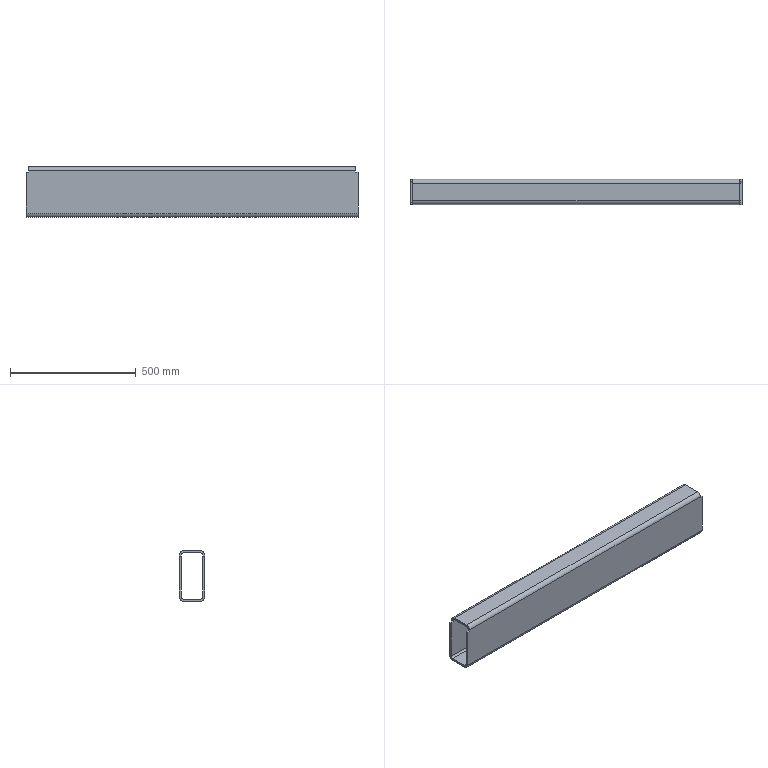Part | SolidWorks | features ICE 1, MirrorPattern 1, WeldMemberFeat 1, WeldmentFeature 1 | 1 solid | 24 faces | box 1321 x 100 x 200 mm | volume 5764189 mm3 | plane 16 | cylinder 8 | commonest cylinder face diameters 16 x4 32 x4
STEP:
#1=CARTESIAN_POINT('',(649.5,50.,84.));
#2=VERTEX_POINT('',#1);
#3=CARTESIAN_POINT('',(649.5,34.,100.));
#4=VERTEX_POINT('',#3);
#5=CARTESIAN_POINT('',(649.5,34.,84.));
#6=DIRECTION('',(1.,0.,0.));
#7=DIRECTION('',(0.,0.,-1.));
#8=AXIS2_PLACEMENT_3D('',#5,#6,#7);
#9=CIRCLE('',#8,16.);
#10=EDGE_CURVE('',#2,#4,#9,.T.);
#11=ORIENTED_EDGE('',*,*,#10,.F.);
#12=CARTESIAN_POINT('',(-649.5,50.,84.));
#13=VERTEX_POINT('',#12);
#14=CARTESIAN_POINT('',(660.5,50.,84.));
#15=DIRECTION('',(-1.,0.,0.));
#16=VECTOR('',#15,1000.);
#17=LINE('',#14,#16);
#18=EDGE_CURVE('',#2,#13,#17,.T.);
#19=ORIENTED_EDGE('',*,*,#18,.T.);
#20=CARTESIAN_POINT('',(-649.5,34.,100.));
#21=VERTEX_POINT('',#20);
#22=CARTESIAN_POINT('',(-649.5,34.,84.));
#23=DIRECTION('',(1.,0.,0.));
#24=DIRECTION('',(0.,0.,-1.));
#25=AXIS2_PLACEMENT_3D('',#22,#23,#24);
#26=CIRCLE('',#25,16.);
#27=EDGE_CURVE('',#13,#21,#26,.T.);
#28=ORIENTED_EDGE('',*,*,#27,.T.);
#29=CARTESIAN_POINT('',(660.5,34.,100.));
#30=DIRECTION('',(-1.,0.,0.));
#31=VECTOR('',#30,1000.);
#32=LINE('',#29,#31);
#33=EDGE_CURVE('',#4,#21,#32,.T.);
#34=ORIENTED_EDGE('',*,*,#33,.F.);
#35=EDGE_LOOP('',(#11,#19,#28,#34));
#36=FACE_OUTER_BOUND('',#35,.T.);
#37=CARTESIAN_POINT('',(660.5,34.,84.));
#38=DIRECTION('',(-1.,0.,0.));
#39=DIRECTION('',(0.,0.,1.));
#40=AXIS2_PLACEMENT_3D('',#37,#38,#39);
#41=CYLINDRICAL_SURFACE('',#40,16.);
#42=ADVANCED_FACE('',(#36),#41,.T.);
#43=CARTESIAN_POINT('',(649.5,-34.,100.));
#44=VERTEX_POINT('',#43);
#45=CARTESIAN_POINT('',(649.5,50.,100.));
#46=DIRECTION('',(0.,-1.,0.));
#47=VECTOR('',#46,1000.);
#48=LINE('',#45,#47);
#49=EDGE_CURVE('',#4,#44,#48,.T.);
#50=ORIENTED_EDGE('',*,*,#49,.F.);
#51=ORIENTED_EDGE('',*,*,#33,.T.);
#52=CARTESIAN_POINT('',(-649.5,-34.,100.));
#53=VERTEX_POINT('',#52);
#54=CARTESIAN_POINT('',(-649.5,50.,100.));
#55=DIRECTION('',(0.,-1.,0.));
#56=VECTOR('',#55,1000.);
#57=LINE('',#54,#56);
#58=EDGE_CURVE('',#21,#53,#57,.T.);
#59=ORIENTED_EDGE('',*,*,#58,.T.);
#60=CARTESIAN_POINT('',(660.5,-34.,100.));
#61=DIRECTION('',(-1.,0.,0.));
#62=VECTOR('',#61,1000.);
#63=LINE('',#60,#62);
#64=EDGE_CURVE('',#44,#53,#63,.T.);
#65=ORIENTED_EDGE('',*,*,#64,.F.);
#66=EDGE_LOOP('',(#50,#51,#59,#65));
#67=FACE_OUTER_BOUND('',#66,.T.);
#68=CARTESIAN_POINT('',(660.5,34.,100.));
#69=DIRECTION('',(0.,0.,-1.));
#70=DIRECTION('',(-1.,0.,0.));
#71=AXIS2_PLACEMENT_3D('',#68,#69,#70);
#72=PLANE('',#71);
#73=ADVANCED_FACE('',(#67),#72,.F.);
#74=CARTESIAN_POINT('',(649.5,-50.,84.));
#75=VERTEX_POINT('',#74);
#76=CARTESIAN_POINT('',(649.5,-34.,84.));
#77=DIRECTION('',(1.,0.,0.));
#78=DIRECTION('',(0.,0.,-1.));
#79=AXIS2_PLACEMENT_3D('',#76,#77,#78);
#80=CIRCLE('',#79,16.);
#81=EDGE_CURVE('',#44,#75,#80,.T.);
#82=ORIENTED_EDGE('',*,*,#81,.F.);
#83=ORIENTED_EDGE('',*,*,#64,.T.);
#84=CARTESIAN_POINT('',(-649.5,-50.,84.));
#85=VERTEX_POINT('',#84);
#86=CARTESIAN_POINT('',(-649.5,-34.,84.));
#87=DIRECTION('',(1.,0.,0.));
#88=DIRECTION('',(0.,0.,-1.));
#89=AXIS2_PLACEMENT_3D('',#86,#87,#88);
#90=CIRCLE('',#89,16.);
#91=EDGE_CURVE('',#53,#85,#90,.T.);
#92=ORIENTED_EDGE('',*,*,#91,.T.);
#93=CARTESIAN_POINT('',(660.5,-50.,84.));
#94=DIRECTION('',(-1.,0.,0.));
#95=VECTOR('',#94,1000.);
#96=LINE('',#93,#95);
#97=EDGE_CURVE('',#75,#85,#96,.T.);
#98=ORIENTED_EDGE('',*,*,#97,.F.);
#99=EDGE_LOOP('',(#82,#83,#92,#98));
#100=FACE_OUTER_BOUND('',#99,.T.);
#101=CARTESIAN_POINT('',(660.5,-34.,84.));
#102=DIRECTION('',(-1.,0.,0.));
#103=DIRECTION('',(0.,0.,1.));
#104=AXIS2_PLACEMENT_3D('',#101,#102,#103);
#105=CYLINDRICAL_SURFACE('',#104,16.);
#106=ADVANCED_FACE('',(#100),#105,.T.);
#107=CARTESIAN_POINT('',(660.5,-50.,78.));
#108=VERTEX_POINT('',#107);
#109=CARTESIAN_POINT('',(649.5,-50.,78.));
#110=VERTEX_POINT('',#109);
#111=CARTESIAN_POINT('',(660.5,-50.,78.));
#112=DIRECTION('',(-1.,0.,0.));
#113=VECTOR('',#112,1000.);
#114=LINE('',#111,#113);
#115=EDGE_CURVE('',#108,#110,#114,.T.);
#116=ORIENTED_EDGE('',*,*,#115,.T.);
#117=CARTESIAN_POINT('',(649.5,-50.,100.));
#118=DIRECTION('',(0.,0.,1.));
#119=VECTOR('',#118,1000.);
#120=LINE('',#117,#119);
#121=EDGE_CURVE('',#110,#75,#120,.T.);
#122=ORIENTED_EDGE('',*,*,#121,.T.);
#123=ORIENTED_EDGE('',*,*,#97,.T.);
#124=CARTESIAN_POINT('',(-649.5,-50.,78.));
#125=VERTEX_POINT('',#124);
#126=CARTESIAN_POINT('',(-649.5,-50.,100.));
#127=DIRECTION('',(0.,0.,1.));
#128=VECTOR('',#127,1000.);
#129=LINE('',#126,#128);
#130=EDGE_CURVE('',#125,#85,#129,.T.);
#131=ORIENTED_EDGE('',*,*,#130,.F.);
#132=CARTESIAN_POINT('',(-660.5,-50.,78.));
#133=VERTEX_POINT('',#132);
#134=CARTESIAN_POINT('',(-660.5,-50.,78.));
#135=DIRECTION('',(1.,0.,0.));
#136=VECTOR('',#135,1000.);
#137=LINE('',#134,#136);
#138=EDGE_CURVE('',#133,#125,#137,.T.);
#139=ORIENTED_EDGE('',*,*,#138,.F.);
#140=CARTESIAN_POINT('',(-660.5,-50.,-84.));
#141=VERTEX_POINT('',#140);
#142=CARTESIAN_POINT('',(-660.5,-50.,-84.));
#143=DIRECTION('',(0.,0.,-1.));
#144=VECTOR('',#143,1000.);
#145=LINE('',#142,#144);
#146=EDGE_CURVE('',#133,#141,#145,.T.);
#147=ORIENTED_EDGE('',*,*,#146,.T.);
#148=CARTESIAN_POINT('',(660.5,-50.,-84.));
#149=VERTEX_POINT('',#148);
#150=CARTESIAN_POINT('',(660.5,-50.,-84.));
#151=DIRECTION('',(-1.,0.,0.));
#152=VECTOR('',#151,1000.);
#153=LINE('',#150,#152);
#154=EDGE_CURVE('',#149,#141,#153,.T.);
#155=ORIENTED_EDGE('',*,*,#154,.F.);
#156=CARTESIAN_POINT('',(660.5,-50.,-84.));
#157=DIRECTION('',(0.,0.,-1.));
#158=VECTOR('',#157,1000.);
#159=LINE('',#156,#158);
#160=EDGE_CURVE('',#108,#149,#159,.T.);
#161=ORIENTED_EDGE('',*,*,#160,.F.);
#162=EDGE_LOOP('',(#116,#122,#123,#131,#139,#147,#155,#161));
#163=FACE_OUTER_BOUND('',#162,.T.);
#164=CARTESIAN_POINT('',(660.5,-50.,-84.));
#165=DIRECTION('',(0.,1.,0.));
#166=DIRECTION('',(0.,0.,1.));
#167=AXIS2_PLACEMENT_3D('',#164,#165,#166);
#168=PLANE('',#167);
#169=ADVANCED_FACE('',(#163),#168,.F.);
#170=CARTESIAN_POINT('',(649.5,-34.,92.));
#171=VERTEX_POINT('',#170);
#172=CARTESIAN_POINT('',(-649.5,-34.,92.));
#173=VERTEX_POINT('',#172);
#174=CARTESIAN_POINT('',(660.5,-34.,92.));
#175=DIRECTION('',(-1.,0.,0.));
#176=VECTOR('',#175,1000.);
#177=LINE('',#174,#176);
#178=EDGE_CURVE('',#171,#173,#177,.T.);
#179=ORIENTED_EDGE('',*,*,#178,.F.);
#180=CARTESIAN_POINT('',(649.5,-42.,84.));
#181=VERTEX_POINT('',#180);
#182=CARTESIAN_POINT('',(649.5,-34.,84.));
#183=DIRECTION('',(1.,0.,0.));
#184=DIRECTION('',(0.,0.,-1.));
#185=AXIS2_PLACEMENT_3D('',#182,#183,#184);
#186=CIRCLE('',#185,8.);
#187=EDGE_CURVE('',#171,#181,#186,.T.);
#188=ORIENTED_EDGE('',*,*,#187,.T.);
#189=CARTESIAN_POINT('',(-649.5,-42.,84.));
#190=VERTEX_POINT('',#189);
#191=CARTESIAN_POINT('',(660.5,-42.,84.));
#192=DIRECTION('',(-1.,0.,0.));
#193=VECTOR('',#192,1000.);
#194=LINE('',#191,#193);
#195=EDGE_CURVE('',#181,#190,#194,.T.);
#196=ORIENTED_EDGE('',*,*,#195,.T.);
#197=CARTESIAN_POINT('',(-649.5,-34.,84.));
#198=DIRECTION('',(1.,0.,0.));
#199=DIRECTION('',(0.,0.,-1.));
#200=AXIS2_PLACEMENT_3D('',#197,#198,#199);
#201=CIRCLE('',#200,8.);
#202=EDGE_CURVE('',#173,#190,#201,.T.);
#203=ORIENTED_EDGE('',*,*,#202,.F.);
#204=EDGE_LOOP('',(#179,#188,#196,#203));
#205=FACE_OUTER_BOUND('',#204,.T.);
#206=CARTESIAN_POINT('',(660.5,-34.,84.));
#207=DIRECTION('',(-1.,0.,0.));
#208=DIRECTION('',(0.,0.,1.));
#209=AXIS2_PLACEMENT_3D('',#206,#207,#208);
#210=CYLINDRICAL_SURFACE('',#209,8.);
#211=ADVANCED_FACE('',(#205),#210,.F.);
#212=CARTESIAN_POINT('',(649.5,34.,92.));
#213=VERTEX_POINT('',#212);
#214=CARTESIAN_POINT('',(-649.5,34.,92.));
#215=VERTEX_POINT('',#214);
#216=CARTESIAN_POINT('',(660.5,34.,92.));
#217=DIRECTION('',(-1.,0.,0.));
#218=VECTOR('',#217,1000.);
#219=LINE('',#216,#218);
#220=EDGE_CURVE('',#213,#215,#219,.T.);
#221=ORIENTED_EDGE('',*,*,#220,.F.);
#222=CARTESIAN_POINT('',(649.5,34.,92.));
#223=DIRECTION('',(0.,-1.,0.));
#224=VECTOR('',#223,1000.);
#225=LINE('',#222,#224);
#226=EDGE_CURVE('',#213,#171,#225,.T.);
#227=ORIENTED_EDGE('',*,*,#226,.T.);
#228=ORIENTED_EDGE('',*,*,#178,.T.);
#229=CARTESIAN_POINT('',(-649.5,34.,92.));
#230=DIRECTION('',(0.,-1.,0.));
#231=VECTOR('',#230,1000.);
#232=LINE('',#229,#231);
#233=EDGE_CURVE('',#215,#173,#232,.T.);
#234=ORIENTED_EDGE('',*,*,#233,.F.);
#235=EDGE_LOOP('',(#221,#227,#228,#234));
#236=FACE_OUTER_BOUND('',#235,.T.);
#237=CARTESIAN_POINT('',(660.5,34.,92.));
#238=DIRECTION('',(0.,0.,-1.));
#239=DIRECTION('',(-1.,0.,0.));
#240=AXIS2_PLACEMENT_3D('',#237,#238,#239);
#241=PLANE('',#240);
#242=ADVANCED_FACE('',(#236),#241,.T.);
#243=CARTESIAN_POINT('',(649.5,42.,84.));
#244=VERTEX_POINT('',#243);
#245=CARTESIAN_POINT('',(-649.5,42.,84.));
#246=VERTEX_POINT('',#245);
#247=CARTESIAN_POINT('',(660.5,42.,84.));
#248=DIRECTION('',(-1.,0.,0.));
#249=VECTOR('',#248,1000.);
#250=LINE('',#247,#249);
#251=EDGE_CURVE('',#244,#246,#250,.T.);
#252=ORIENTED_EDGE('',*,*,#251,.F.);
#253=CARTESIAN_POINT('',(649.5,34.,84.));
#254=DIRECTION('',(1.,0.,0.));
#255=DIRECTION('',(0.,0.,-1.));
#256=AXIS2_PLACEMENT_3D('',#253,#254,#255);
#257=CIRCLE('',#256,8.);
#258=EDGE_CURVE('',#244,#213,#257,.T.);
#259=ORIENTED_EDGE('',*,*,#258,.T.);
#260=ORIENTED_EDGE('',*,*,#220,.T.);
#261=CARTESIAN_POINT('',(-649.5,34.,84.));
#262=DIRECTION('',(1.,0.,0.));
#263=DIRECTION('',(0.,0.,-1.));
#264=AXIS2_PLACEMENT_3D('',#261,#262,#263);
#265=CIRCLE('',#264,8.);
#266=EDGE_CURVE('',#246,#215,#265,.T.);
#267=ORIENTED_EDGE('',*,*,#266,.F.);
#268=EDGE_LOOP('',(#252,#259,#260,#267));
#269=FACE_OUTER_BOUND('',#268,.T.);
#270=CARTESIAN_POINT('',(660.5,34.,84.));
#271=DIRECTION('',(-1.,0.,0.));
#272=DIRECTION('',(0.,0.,1.));
#273=AXIS2_PLACEMENT_3D('',#270,#271,#272);
#274=CYLINDRICAL_SURFACE('',#273,8.);
#275=ADVANCED_FACE('',(#269),#274,.F.);
#276=CARTESIAN_POINT('',(660.5,42.,-84.));
#277=VERTEX_POINT('',#276);
#278=CARTESIAN_POINT('',(660.5,42.,78.));
#279=VERTEX_POINT('',#278);
#280=CARTESIAN_POINT('',(660.5,42.,84.));
#281=DIRECTION('',(0.,0.,1.));
#282=VECTOR('',#281,1000.);
#283=LINE('',#280,#282);
#284=EDGE_CURVE('',#277,#279,#283,.T.);
#285=ORIENTED_EDGE('',*,*,#284,.T.);
#286=CARTESIAN_POINT('',(649.5,42.,78.));
#287=VERTEX_POINT('',#286);
#288=CARTESIAN_POINT('',(660.5,42.,78.));
#289=DIRECTION('',(-1.,0.,0.));
#290=VECTOR('',#289,1000.);
#291=LINE('',#288,#290);
#292=EDGE_CURVE('',#279,#287,#291,.T.);
#293=ORIENTED_EDGE('',*,*,#292,.T.);
#294=CARTESIAN_POINT('',(649.5,42.,84.));
#295=DIRECTION('',(0.,0.,1.));
#296=VECTOR('',#295,1000.);
#297=LINE('',#294,#296);
#298=EDGE_CURVE('',#287,#244,#297,.T.);
#299=ORIENTED_EDGE('',*,*,#298,.T.);
#300=ORIENTED_EDGE('',*,*,#251,.T.);
#301=CARTESIAN_POINT('',(-649.5,42.,78.));
#302=VERTEX_POINT('',#301);
#303=CARTESIAN_POINT('',(-649.5,42.,84.));
#304=DIRECTION('',(0.,0.,1.));
#305=VECTOR('',#304,1000.);
#306=LINE('',#303,#305);
#307=EDGE_CURVE('',#302,#246,#306,.T.);
#308=ORIENTED_EDGE('',*,*,#307,.F.);
#309=CARTESIAN_POINT('',(-660.5,42.,78.));
#310=VERTEX_POINT('',#309);
#311=CARTESIAN_POINT('',(660.5,42.,78.));
#312=DIRECTION('',(1.,0.,0.));
#313=VECTOR('',#312,1000.);
#314=LINE('',#311,#313);
#315=EDGE_CURVE('',#310,#302,#314,.T.);
#316=ORIENTED_EDGE('',*,*,#315,.F.);
#317=CARTESIAN_POINT('',(-660.5,42.,-84.));
#318=VERTEX_POINT('',#317);
#319=CARTESIAN_POINT('',(-660.5,42.,84.));
#320=DIRECTION('',(0.,0.,1.));
#321=VECTOR('',#320,1000.);
#322=LINE('',#319,#321);
#323=EDGE_CURVE('',#318,#310,#322,.T.);
#324=ORIENTED_EDGE('',*,*,#323,.F.);
#325=CARTESIAN_POINT('',(660.5,42.,-84.));
#326=DIRECTION('',(-1.,0.,0.));
#327=VECTOR('',#326,1000.);
#328=LINE('',#325,#327);
#329=EDGE_CURVE('',#277,#318,#328,.T.);
#330=ORIENTED_EDGE('',*,*,#329,.F.);
#331=EDGE_LOOP('',(#285,#293,#299,#300,#308,#316,#324,#330));
#332=FACE_OUTER_BOUND('',#331,.T.);
#333=CARTESIAN_POINT('',(660.5,42.,84.));
#334=DIRECTION('',(0.,-1.,0.));
#335=DIRECTION('',(0.,0.,-1.));
#336=AXIS2_PLACEMENT_3D('',#333,#334,#335);
#337=PLANE('',#336);
#338=ADVANCED_FACE('',(#332),#337,.T.);
#339=CARTESIAN_POINT('',(649.5,-42.,78.));
#340=VERTEX_POINT('',#339);
#341=CARTESIAN_POINT('',(649.5,-42.,-84.));
#342=DIRECTION('',(0.,0.,-1.));
#343=VECTOR('',#342,1000.);
#344=LINE('',#341,#343);
#345=EDGE_CURVE('',#181,#340,#344,.T.);
#346=ORIENTED_EDGE('',*,*,#345,.T.);
#347=CARTESIAN_POINT('',(660.5,-42.,78.));
#348=VERTEX_POINT('',#347);
#349=CARTESIAN_POINT('',(660.5,-42.,78.));
#350=DIRECTION('',(1.,0.,0.));
#351=VECTOR('',#350,1000.);
#352=LINE('',#349,#351);
#353=EDGE_CURVE('',#340,#348,#352,.T.);
#354=ORIENTED_EDGE('',*,*,#353,.T.);
#355=CARTESIAN_POINT('',(660.5,-42.,-84.));
#356=VERTEX_POINT('',#355);
#357=CARTESIAN_POINT('',(660.5,-42.,-84.));
#358=DIRECTION('',(0.,0.,-1.));
#359=VECTOR('',#358,1000.);
#360=LINE('',#357,#359);
#361=EDGE_CURVE('',#348,#356,#360,.T.);
#362=ORIENTED_EDGE('',*,*,#361,.T.);
#363=CARTESIAN_POINT('',(-660.5,-42.,-84.));
#364=VERTEX_POINT('',#363);
#365=CARTESIAN_POINT('',(660.5,-42.,-84.));
#366=DIRECTION('',(-1.,0.,0.));
#367=VECTOR('',#366,1000.);
#368=LINE('',#365,#367);
#369=EDGE_CURVE('',#356,#364,#368,.T.);
#370=ORIENTED_EDGE('',*,*,#369,.T.);
#371=CARTESIAN_POINT('',(-660.5,-42.,78.));
#372=VERTEX_POINT('',#371);
#373=CARTESIAN_POINT('',(-660.5,-42.,-84.));
#374=DIRECTION('',(0.,0.,-1.));
#375=VECTOR('',#374,1000.);
#376=LINE('',#373,#375);
#377=EDGE_CURVE('',#372,#364,#376,.T.);
#378=ORIENTED_EDGE('',*,*,#377,.F.);
#379=CARTESIAN_POINT('',(-649.5,-42.,78.));
#380=VERTEX_POINT('',#379);
#381=CARTESIAN_POINT('',(660.5,-42.,78.));
#382=DIRECTION('',(-1.,0.,0.));
#383=VECTOR('',#382,1000.);
#384=LINE('',#381,#383);
#385=EDGE_CURVE('',#380,#372,#384,.T.);
#386=ORIENTED_EDGE('',*,*,#385,.F.);
#387=CARTESIAN_POINT('',(-649.5,-42.,-84.));
#388=DIRECTION('',(0.,0.,-1.));
#389=VECTOR('',#388,1000.);
#390=LINE('',#387,#389);
#391=EDGE_CURVE('',#190,#380,#390,.T.);
#392=ORIENTED_EDGE('',*,*,#391,.F.);
#393=ORIENTED_EDGE('',*,*,#195,.F.);
#394=EDGE_LOOP('',(#346,#354,#362,#370,#378,#386,#392,#393));
#395=FACE_OUTER_BOUND('',#394,.T.);
#396=CARTESIAN_POINT('',(660.5,-42.,-84.));
#397=DIRECTION('',(0.,1.,0.));
#398=DIRECTION('',(0.,0.,1.));
#399=AXIS2_PLACEMENT_3D('',#396,#397,#398);
#400=PLANE('',#399);
#401=ADVANCED_FACE('',(#395),#400,.T.);
#402=CARTESIAN_POINT('',(660.5,50.,78.));
#403=VERTEX_POINT('',#402);
#404=CARTESIAN_POINT('',(649.5,50.,78.));
#405=VERTEX_POINT('',#404);
#406=CARTESIAN_POINT('',(660.5,50.,78.));
#407=DIRECTION('',(-1.,0.,0.));
#408=VECTOR('',#407,1000.);
#409=LINE('',#406,#408);
#410=EDGE_CURVE('',#403,#405,#409,.T.);
#411=ORIENTED_EDGE('',*,*,#410,.F.);
#412=CARTESIAN_POINT('',(660.5,50.,-84.));
#413=VERTEX_POINT('',#412);
#414=CARTESIAN_POINT('',(660.5,50.,84.));
#415=DIRECTION('',(0.,0.,1.));
#416=VECTOR('',#415,1000.);
#417=LINE('',#414,#416);
#418=EDGE_CURVE('',#413,#403,#417,.T.);
#419=ORIENTED_EDGE('',*,*,#418,.F.);
#420=CARTESIAN_POINT('',(-660.5,50.,-84.));
#421=VERTEX_POINT('',#420);
#422=CARTESIAN_POINT('',(660.5,50.,-84.));
#423=DIRECTION('',(-1.,0.,0.));
#424=VECTOR('',#423,1000.);
#425=LINE('',#422,#424);
#426=EDGE_CURVE('',#413,#421,#425,.T.);
#427=ORIENTED_EDGE('',*,*,#426,.T.);
#428=CARTESIAN_POINT('',(-660.5,50.,78.));
#429=VERTEX_POINT('',#428);
#430=CARTESIAN_POINT('',(-660.5,50.,84.));
#431=DIRECTION('',(0.,0.,1.));
#432=VECTOR('',#431,1000.);
#433=LINE('',#430,#432);
#434=EDGE_CURVE('',#421,#429,#433,.T.);
#435=ORIENTED_EDGE('',*,*,#434,.T.);
#436=CARTESIAN_POINT('',(-649.5,50.,78.));
#437=VERTEX_POINT('',#436);
#438=CARTESIAN_POINT('',(-660.5,50.,78.));
#439=DIRECTION('',(1.,0.,0.));
#440=VECTOR('',#439,1000.);
#441=LINE('',#438,#440);
#442=EDGE_CURVE('',#429,#437,#441,.T.);
#443=ORIENTED_EDGE('',*,*,#442,.T.);
#444=CARTESIAN_POINT('',(-649.5,50.,100.));
#445=DIRECTION('',(0.,0.,1.));
#446=VECTOR('',#445,1000.);
#447=LINE('',#444,#446);
#448=EDGE_CURVE('',#437,#13,#447,.T.);
#449=ORIENTED_EDGE('',*,*,#448,.T.);
#450=ORIENTED_EDGE('',*,*,#18,.F.);
#451=CARTESIAN_POINT('',(649.5,50.,100.));
#452=DIRECTION('',(0.,0.,1.));
#453=VECTOR('',#452,1000.);
#454=LINE('',#451,#453);
#455=EDGE_CURVE('',#405,#2,#454,.T.);
#456=ORIENTED_EDGE('',*,*,#455,.F.);
#457=EDGE_LOOP('',(#411,#419,#427,#435,#443,#449,#450,#456));
#458=FACE_OUTER_BOUND('',#457,.T.);
#459=CARTESIAN_POINT('',(660.5,50.,84.));
#460=DIRECTION('',(0.,-1.,0.));
#461=DIRECTION('',(0.,0.,-1.));
#462=AXIS2_PLACEMENT_3D('',#459,#460,#461);
#463=PLANE('',#462);
#464=ADVANCED_FACE('',(#458),#463,.F.);
#465=ORIENTED_EDGE('',*,*,#418,.T.);
#466=CARTESIAN_POINT('',(660.5,50.,78.));
#467=DIRECTION('',(0.,-1.,0.));
#468=VECTOR('',#467,1000.);
#469=LINE('',#466,#468);
#470=EDGE_CURVE('',#403,#279,#469,.T.);
#471=ORIENTED_EDGE('',*,*,#470,.T.);
#472=ORIENTED_EDGE('',*,*,#284,.F.);
#473=CARTESIAN_POINT('',(660.5,34.,-92.));
#474=VERTEX_POINT('',#473);
#475=CARTESIAN_POINT('',(660.5,34.,-84.));
#476=DIRECTION('',(1.,0.,0.));
#477=DIRECTION('',(0.,0.,-1.));
#478=AXIS2_PLACEMENT_3D('',#475,#476,#477);
#479=CIRCLE('',#478,8.);
#480=EDGE_CURVE('',#474,#277,#479,.T.);
#481=ORIENTED_EDGE('',*,*,#480,.F.);
#482=CARTESIAN_POINT('',(660.5,-34.,-92.));
#483=VERTEX_POINT('',#482);
#484=CARTESIAN_POINT('',(660.5,-34.,-92.));
#485=DIRECTION('',(0.,1.,0.));
#486=VECTOR('',#485,1000.);
#487=LINE('',#484,#486);
#488=EDGE_CURVE('',#483,#474,#487,.T.);
#489=ORIENTED_EDGE('',*,*,#488,.F.);
#490=CARTESIAN_POINT('',(660.5,-34.,-84.));
#491=DIRECTION('',(1.,0.,0.));
#492=DIRECTION('',(0.,0.,-1.));
#493=AXIS2_PLACEMENT_3D('',#490,#491,#492);
#494=CIRCLE('',#493,8.);
#495=EDGE_CURVE('',#356,#483,#494,.T.);
#496=ORIENTED_EDGE('',*,*,#495,.F.);
#497=ORIENTED_EDGE('',*,*,#361,.F.);
#498=CARTESIAN_POINT('',(660.5,34.,78.));
#499=DIRECTION('',(0.,-1.,0.));
#500=VECTOR('',#499,1000.);
#501=LINE('',#498,#500);
#502=EDGE_CURVE('',#348,#108,#501,.T.);
#503=ORIENTED_EDGE('',*,*,#502,.T.);
#504=ORIENTED_EDGE('',*,*,#160,.T.);
#505=CARTESIAN_POINT('',(660.5,-34.,-100.));
#506=VERTEX_POINT('',#505);
#507=CARTESIAN_POINT('',(660.5,-34.,-84.));
#508=DIRECTION('',(1.,0.,0.));
#509=DIRECTION('',(0.,0.,-1.));
#510=AXIS2_PLACEMENT_3D('',#507,#508,#509);
#511=CIRCLE('',#510,16.);
#512=EDGE_CURVE('',#149,#506,#511,.T.);
#513=ORIENTED_EDGE('',*,*,#512,.T.);
#514=CARTESIAN_POINT('',(660.5,34.,-100.));
#515=VERTEX_POINT('',#514);
#516=CARTESIAN_POINT('',(660.5,-34.,-100.));
#517=DIRECTION('',(0.,1.,0.));
#518=VECTOR('',#517,1000.);
#519=LINE('',#516,#518);
#520=EDGE_CURVE('',#506,#515,#519,.T.);
#521=ORIENTED_EDGE('',*,*,#520,.T.);
#522=CARTESIAN_POINT('',(660.5,34.,-84.));
#523=DIRECTION('',(1.,0.,0.));
#524=DIRECTION('',(0.,0.,-1.));
#525=AXIS2_PLACEMENT_3D('',#522,#523,#524);
#526=CIRCLE('',#525,16.);
#527=EDGE_CURVE('',#515,#413,#526,.T.);
#528=ORIENTED_EDGE('',*,*,#527,.T.);
#529=EDGE_LOOP('',(#465,#471,#472,#481,#489,#496,#497,#503,#504,#513,#521,#528));
#530=FACE_OUTER_BOUND('',#529,.T.);
#531=CARTESIAN_POINT('',(660.5,34.,84.));
#532=DIRECTION('',(1.,0.,0.));
#533=DIRECTION('',(0.,0.,-1.));
#534=AXIS2_PLACEMENT_3D('',#531,#532,#533);
#535=PLANE('',#534);
#536=ADVANCED_FACE('',(#530),#535,.T.);
#537=CARTESIAN_POINT('',(-660.5,-34.,-100.));
#538=VERTEX_POINT('',#537);
#539=CARTESIAN_POINT('',(-660.5,-34.,-84.));
#540=DIRECTION('',(1.,0.,0.));
#541=DIRECTION('',(0.,0.,-1.));
#542=AXIS2_PLACEMENT_3D('',#539,#540,#541);
#543=CIRCLE('',#542,16.);
#544=EDGE_CURVE('',#141,#538,#543,.T.);
#545=ORIENTED_EDGE('',*,*,#544,.T.);
#546=CARTESIAN_POINT('',(660.5,-34.,-100.));
#547=DIRECTION('',(-1.,0.,0.));
#548=VECTOR('',#547,1000.);
#549=LINE('',#546,#548);
#550=EDGE_CURVE('',#506,#538,#549,.T.);
#551=ORIENTED_EDGE('',*,*,#550,.F.);
#552=ORIENTED_EDGE('',*,*,#512,.F.);
#553=ORIENTED_EDGE('',*,*,#154,.T.);
#554=EDGE_LOOP('',(#545,#551,#552,#553));
#555=FACE_OUTER_BOUND('',#554,.T.);
#556=CARTESIAN_POINT('',(660.5,-34.,-84.));
#557=DIRECTION('',(-1.,0.,0.));
#558=DIRECTION('',(0.,0.,1.));
#559=AXIS2_PLACEMENT_3D('',#556,#557,#558);
#560=CYLINDRICAL_SURFACE('',#559,16.);
#561=ADVANCED_FACE('',(#555),#560,.T.);
#562=CARTESIAN_POINT('',(-660.5,34.,-100.));
#563=VERTEX_POINT('',#562);
#564=CARTESIAN_POINT('',(-660.5,-34.,-100.));
#565=DIRECTION('',(0.,1.,0.));
#566=VECTOR('',#565,1000.);
#567=LINE('',#564,#566);
#568=EDGE_CURVE('',#538,#563,#567,.T.);
#569=ORIENTED_EDGE('',*,*,#568,.T.);
#570=CARTESIAN_POINT('',(660.5,34.,-100.));
#571=DIRECTION('',(-1.,0.,0.));
#572=VECTOR('',#571,1000.);
#573=LINE('',#570,#572);
#574=EDGE_CURVE('',#515,#563,#573,.T.);
#575=ORIENTED_EDGE('',*,*,#574,.F.);
#576=ORIENTED_EDGE('',*,*,#520,.F.);
#577=ORIENTED_EDGE('',*,*,#550,.T.);
#578=EDGE_LOOP('',(#569,#575,#576,#577));
#579=FACE_OUTER_BOUND('',#578,.T.);
#580=CARTESIAN_POINT('',(660.5,-34.,-100.));
#581=DIRECTION('',(0.,0.,1.));
#582=DIRECTION('',(1.,0.,0.));
#583=AXIS2_PLACEMENT_3D('',#580,#581,#582);
#584=PLANE('',#583);
#585=ADVANCED_FACE('',(#579),#584,.F.);
#586=CARTESIAN_POINT('',(-660.5,34.,-84.));
#587=DIRECTION('',(1.,0.,0.));
#588=DIRECTION('',(0.,0.,-1.));
#589=AXIS2_PLACEMENT_3D('',#586,#587,#588);
#590=CIRCLE('',#589,16.);
#591=EDGE_CURVE('',#563,#421,#590,.T.);
#592=ORIENTED_EDGE('',*,*,#591,.T.);
#593=ORIENTED_EDGE('',*,*,#426,.F.);
#594=ORIENTED_EDGE('',*,*,#527,.F.);
#595=ORIENTED_EDGE('',*,*,#574,.T.);
#596=EDGE_LOOP('',(#592,#593,#594,#595));
#597=FACE_OUTER_BOUND('',#596,.T.);
#598=CARTESIAN_POINT('',(660.5,34.,-84.));
#599=DIRECTION('',(-1.,0.,0.));
#600=DIRECTION('',(0.,0.,1.));
#601=AXIS2_PLACEMENT_3D('',#598,#599,#600);
#602=CYLINDRICAL_SURFACE('',#601,16.);
#603=ADVANCED_FACE('',(#597),#602,.T.);
#604=CARTESIAN_POINT('',(-660.5,34.,-92.));
#605=VERTEX_POINT('',#604);
#606=CARTESIAN_POINT('',(-660.5,34.,-84.));
#607=DIRECTION('',(1.,0.,0.));
#608=DIRECTION('',(0.,0.,-1.));
#609=AXIS2_PLACEMENT_3D('',#606,#607,#608);
#610=CIRCLE('',#609,8.);
#611=EDGE_CURVE('',#605,#318,#610,.T.);
#612=ORIENTED_EDGE('',*,*,#611,.F.);
#613=CARTESIAN_POINT('',(660.5,34.,-92.));
#614=DIRECTION('',(-1.,0.,0.));
#615=VECTOR('',#614,1000.);
#616=LINE('',#613,#615);
#617=EDGE_CURVE('',#474,#605,#616,.T.);
#618=ORIENTED_EDGE('',*,*,#617,.F.);
#619=ORIENTED_EDGE('',*,*,#480,.T.);
#620=ORIENTED_EDGE('',*,*,#329,.T.);
#621=EDGE_LOOP('',(#612,#618,#619,#620));
#622=FACE_OUTER_BOUND('',#621,.T.);
#623=CARTESIAN_POINT('',(660.5,34.,-84.));
#624=DIRECTION('',(-1.,0.,0.));
#625=DIRECTION('',(0.,0.,1.));
#626=AXIS2_PLACEMENT_3D('',#623,#624,#625);
#627=CYLINDRICAL_SURFACE('',#626,8.);
#628=ADVANCED_FACE('',(#622),#627,.F.);
#629=CARTESIAN_POINT('',(-660.5,-34.,-92.));
#630=VERTEX_POINT('',#629);
#631=CARTESIAN_POINT('',(-660.5,-34.,-92.));
#632=DIRECTION('',(0.,1.,0.));
#633=VECTOR('',#632,1000.);
#634=LINE('',#631,#633);
#635=EDGE_CURVE('',#630,#605,#634,.T.);
#636=ORIENTED_EDGE('',*,*,#635,.F.);
#637=CARTESIAN_POINT('',(660.5,-34.,-92.));
#638=DIRECTION('',(-1.,0.,0.));
#639=VECTOR('',#638,1000.);
#640=LINE('',#637,#639);
#641=EDGE_CURVE('',#483,#630,#640,.T.);
#642=ORIENTED_EDGE('',*,*,#641,.F.);
#643=ORIENTED_EDGE('',*,*,#488,.T.);
#644=ORIENTED_EDGE('',*,*,#617,.T.);
#645=EDGE_LOOP('',(#636,#642,#643,#644));
#646=FACE_OUTER_BOUND('',#645,.T.);
#647=CARTESIAN_POINT('',(660.5,-34.,-92.));
#648=DIRECTION('',(0.,0.,1.));
#649=DIRECTION('',(1.,0.,0.));
#650=AXIS2_PLACEMENT_3D('',#647,#648,#649);
#651=PLANE('',#650);
#652=ADVANCED_FACE('',(#646),#651,.T.);
#653=CARTESIAN_POINT('',(-660.5,-34.,-84.));
#654=DIRECTION('',(1.,0.,0.));
#655=DIRECTION('',(0.,0.,-1.));
#656=AXIS2_PLACEMENT_3D('',#653,#654,#655);
#657=CIRCLE('',#656,8.);
#658=EDGE_CURVE('',#364,#630,#657,.T.);
#659=ORIENTED_EDGE('',*,*,#658,.F.);
#660=ORIENTED_EDGE('',*,*,#369,.F.);
#661=ORIENTED_EDGE('',*,*,#495,.T.);
#662=ORIENTED_EDGE('',*,*,#641,.T.);
#663=EDGE_LOOP('',(#659,#660,#661,#662));
#664=FACE_OUTER_BOUND('',#663,.T.);
#665=CARTESIAN_POINT('',(660.5,-34.,-84.));
#666=DIRECTION('',(-1.,0.,0.));
#667=DIRECTION('',(0.,0.,1.));
#668=AXIS2_PLACEMENT_3D('',#665,#666,#667);
#669=CYLINDRICAL_SURFACE('',#668,8.);
#670=ADVANCED_FACE('',(#664),#669,.F.);
#671=ORIENTED_EDGE('',*,*,#146,.F.);
#672=CARTESIAN_POINT('',(-660.5,34.,78.));
#673=DIRECTION('',(0.,1.,0.));
#674=VECTOR('',#673,1000.);
#675=LINE('',#672,#674);
#676=EDGE_CURVE('',#133,#372,#675,.T.);
#677=ORIENTED_EDGE('',*,*,#676,.T.);
#678=ORIENTED_EDGE('',*,*,#377,.T.);
#679=ORIENTED_EDGE('',*,*,#658,.T.);
#680=ORIENTED_EDGE('',*,*,#635,.T.);
#681=ORIENTED_EDGE('',*,*,#611,.T.);
#682=ORIENTED_EDGE('',*,*,#323,.T.);
#683=CARTESIAN_POINT('',(-660.5,50.,78.));
#684=DIRECTION('',(0.,-1.,0.));
#685=VECTOR('',#684,1000.);
#686=LINE('',#683,#685);
#687=EDGE_CURVE('',#429,#310,#686,.T.);
#688=ORIENTED_EDGE('',*,*,#687,.F.);
#689=ORIENTED_EDGE('',*,*,#434,.F.);
#690=ORIENTED_EDGE('',*,*,#591,.F.);
#691=ORIENTED_EDGE('',*,*,#568,.F.);
#692=ORIENTED_EDGE('',*,*,#544,.F.);
#693=EDGE_LOOP('',(#671,#677,#678,#679,#680,#681,#682,#688,#689,#690,#691,#692));
#694=FACE_OUTER_BOUND('',#693,.T.);
#695=CARTESIAN_POINT('',(-660.5,34.,84.));
#696=DIRECTION('',(1.,0.,0.));
#697=DIRECTION('',(0.,0.,-1.));
#698=AXIS2_PLACEMENT_3D('',#695,#696,#697);
#699=PLANE('',#698);
#700=ADVANCED_FACE('',(#694),#699,.F.);
#701=ORIENTED_EDGE('',*,*,#448,.F.);
#702=CARTESIAN_POINT('',(-649.5,50.,78.));
#703=DIRECTION('',(0.,-1.,0.));
#704=VECTOR('',#703,1000.);
#705=LINE('',#702,#704);
#706=EDGE_CURVE('',#437,#302,#705,.T.);
#707=ORIENTED_EDGE('',*,*,#706,.T.);
#708=ORIENTED_EDGE('',*,*,#307,.T.);
#709=ORIENTED_EDGE('',*,*,#266,.T.);
#710=ORIENTED_EDGE('',*,*,#233,.T.);
#711=ORIENTED_EDGE('',*,*,#202,.T.);
#712=ORIENTED_EDGE('',*,*,#391,.T.);
#713=CARTESIAN_POINT('',(-649.5,50.,78.));
#714=DIRECTION('',(0.,-1.,0.));
#715=VECTOR('',#714,1000.);
#716=LINE('',#713,#715);
#717=EDGE_CURVE('',#380,#125,#716,.T.);
#718=ORIENTED_EDGE('',*,*,#717,.T.);
#719=ORIENTED_EDGE('',*,*,#130,.T.);
#720=ORIENTED_EDGE('',*,*,#91,.F.);
#721=ORIENTED_EDGE('',*,*,#58,.F.);
#722=ORIENTED_EDGE('',*,*,#27,.F.);
#723=EDGE_LOOP('',(#701,#707,#708,#709,#710,#711,#712,#718,#719,#720,#721,#722));
#724=FACE_OUTER_BOUND('',#723,.T.);
#725=CARTESIAN_POINT('',(-649.5,50.,100.));
#726=DIRECTION('',(1.,0.,0.));
#727=DIRECTION('',(0.,0.,-1.));
#728=AXIS2_PLACEMENT_3D('',#725,#726,#727);
#729=PLANE('',#728);
#730=ADVANCED_FACE('',(#724),#729,.F.);
#731=ORIENTED_EDGE('',*,*,#315,.T.);
#732=ORIENTED_EDGE('',*,*,#706,.F.);
#733=ORIENTED_EDGE('',*,*,#442,.F.);
#734=ORIENTED_EDGE('',*,*,#687,.T.);
#735=EDGE_LOOP('',(#731,#732,#733,#734));
#736=FACE_OUTER_BOUND('',#735,.T.);
#737=CARTESIAN_POINT('',(-660.5,50.,78.));
#738=DIRECTION('',(0.,0.,-1.));
#739=DIRECTION('',(-1.,0.,0.));
#740=AXIS2_PLACEMENT_3D('',#737,#738,#739);
#741=PLANE('',#740);
#742=ADVANCED_FACE('',(#736),#741,.F.);
#743=ORIENTED_EDGE('',*,*,#385,.T.);
#744=ORIENTED_EDGE('',*,*,#676,.F.);
#745=ORIENTED_EDGE('',*,*,#138,.T.);
#746=ORIENTED_EDGE('',*,*,#717,.F.);
#747=EDGE_LOOP('',(#743,#744,#745,#746));
#748=FACE_OUTER_BOUND('',#747,.T.);
#749=CARTESIAN_POINT('',(-660.5,50.,78.));
#750=DIRECTION('',(0.,0.,-1.));
#751=DIRECTION('',(-1.,0.,0.));
#752=AXIS2_PLACEMENT_3D('',#749,#750,#751);
#753=PLANE('',#752);
#754=ADVANCED_FACE('',(#748),#753,.F.);
#755=ORIENTED_EDGE('',*,*,#10,.T.);
#756=ORIENTED_EDGE('',*,*,#49,.T.);
#757=ORIENTED_EDGE('',*,*,#81,.T.);
#758=ORIENTED_EDGE('',*,*,#121,.F.);
#759=CARTESIAN_POINT('',(649.5,50.,78.));
#760=DIRECTION('',(0.,-1.,0.));
#761=VECTOR('',#760,1000.);
#762=LINE('',#759,#761);
#763=EDGE_CURVE('',#340,#110,#762,.T.);
#764=ORIENTED_EDGE('',*,*,#763,.F.);
#765=ORIENTED_EDGE('',*,*,#345,.F.);
#766=ORIENTED_EDGE('',*,*,#187,.F.);
#767=ORIENTED_EDGE('',*,*,#226,.F.);
#768=ORIENTED_EDGE('',*,*,#258,.F.);
#769=ORIENTED_EDGE('',*,*,#298,.F.);
#770=CARTESIAN_POINT('',(649.5,50.,78.));
#771=DIRECTION('',(0.,-1.,0.));
#772=VECTOR('',#771,1000.);
#773=LINE('',#770,#772);
#774=EDGE_CURVE('',#405,#287,#773,.T.);
#775=ORIENTED_EDGE('',*,*,#774,.F.);
#776=ORIENTED_EDGE('',*,*,#455,.T.);
#777=EDGE_LOOP('',(#755,#756,#757,#758,#764,#765,#766,#767,#768,#769,#775,#776));
#778=FACE_OUTER_BOUND('',#777,.T.);
#779=CARTESIAN_POINT('',(649.5,50.,100.));
#780=DIRECTION('',(1.,0.,0.));
#781=DIRECTION('',(0.,0.,-1.));
#782=AXIS2_PLACEMENT_3D('',#779,#780,#781);
#783=PLANE('',#782);
#784=ADVANCED_FACE('',(#778),#783,.T.);
#785=ORIENTED_EDGE('',*,*,#470,.F.);
#786=ORIENTED_EDGE('',*,*,#410,.T.);
#787=ORIENTED_EDGE('',*,*,#774,.T.);
#788=ORIENTED_EDGE('',*,*,#292,.F.);
#789=EDGE_LOOP('',(#785,#786,#787,#788));
#790=FACE_OUTER_BOUND('',#789,.T.);
#791=CARTESIAN_POINT('',(660.5,50.,78.));
#792=DIRECTION('',(0.,0.,1.));
#793=DIRECTION('',(1.,0.,0.));
#794=AXIS2_PLACEMENT_3D('',#791,#792,#793);
#795=PLANE('',#794);
#796=ADVANCED_FACE('',(#790),#795,.T.);
#797=ORIENTED_EDGE('',*,*,#763,.T.);
#798=ORIENTED_EDGE('',*,*,#115,.F.);
#799=ORIENTED_EDGE('',*,*,#502,.F.);
#800=ORIENTED_EDGE('',*,*,#353,.F.);
#801=EDGE_LOOP('',(#797,#798,#799,#800));
#802=FACE_OUTER_BOUND('',#801,.T.);
#803=CARTESIAN_POINT('',(660.5,50.,78.));
#804=DIRECTION('',(0.,0.,1.));
#805=DIRECTION('',(1.,0.,0.));
#806=AXIS2_PLACEMENT_3D('',#803,#804,#805);
#807=PLANE('',#806);
#808=ADVANCED_FACE('',(#802),#807,.T.);
#809=CLOSED_SHELL('',(#42,#73,#106,#169,#211,#242,#275,#338,#401,#464,#536,#561,#585,#603,#628,#652,#670,#700,#730,#742,#754,#784,#796,#808));
#810=MANIFOLD_SOLID_BREP('',#809);
#811=CARTESIAN_POINT('',(0.,0.,0.));
#812=DIRECTION('',(0.,0.,1.));
#813=DIRECTION('',(1.,0.,0.));
#814=AXIS2_PLACEMENT_3D('',#811,#812,#813);
#815=(LENGTH_UNIT()NAMED_UNIT(*)SI_UNIT(.MILLI.,.METRE.));
#816=UNCERTAINTY_MEASURE_WITH_UNIT(LENGTH_MEASURE(0.00001),#815,'','');
#817=(NAMED_UNIT(*)PLANE_ANGLE_UNIT()SI_UNIT($,.RADIAN.));
#818=(NAMED_UNIT(*)SI_UNIT($,.STERADIAN.)SOLID_ANGLE_UNIT());
#819=(GEOMETRIC_REPRESENTATION_CONTEXT(3)GLOBAL_UNCERTAINTY_ASSIGNED_CONTEXT((#816))GLOBAL_UNIT_ASSIGNED_CONTEXT((#815,#817,#818))REPRESENTATION_CONTEXT('',''));
#820=ADVANCED_BREP_SHAPE_REPRESENTATION('',(#810,#814),#819);